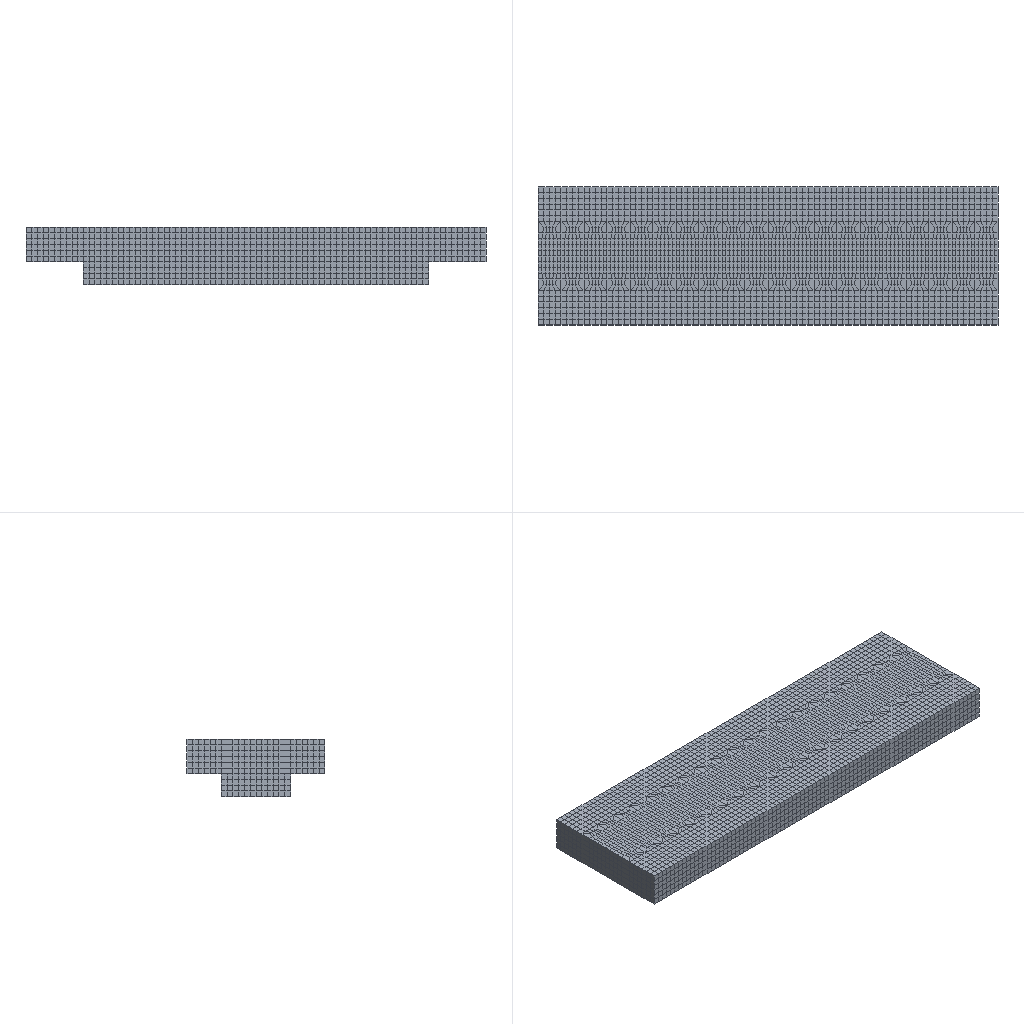Simulation study | abaqus
Set-up summary:
category,name,step,type,value,unit,region
solver,abaqus
solver,version,,,Abaqus/Standard 2020
units,not stated in the deck,,not stated
analysis,deck,,coupled temperature-displacement,coupled temperature-displacement
load_step,Step-1,Step-1,coupled temperature-displacement,nlgeom=True
contact,interactions,,,general=0 pairs=1 ties=0
load_step,requested,,,1
mesh,nodes,,,20926
mesh,elements,,,16800
element_type,C3D8RT,,solid,16800
load,load commands in deck,,count,4
bc,support commands in deck,,count,8
material,TC4,,in results
check,setup vs results,,match,"per instance, exact: element labels, types and connectivity; labels of the nodes the elements use; coordinates of those nodes at SINGLE_PRECISION in 2 of 2 instance(s)"
Abaqus input file, long lists of numbers shortened:
*Heading
** Job name: Job-1 Model name: Model-1
** Generated by: Abaqus/CAE 2020
*Preprint, echo=NO, model=NO, history=NO, contact=NO
**
** PARTS
**
*Part, name=Part-1
*Node
      1,           0.,          -9.,           3.
      2,           0.,        -8.25,           3.
** (3963 more lines like these left out)
*Element, type=C3D8RT
   1,   66,   67,   80,   79,    1,    2,   15,   14
   2,   67,   68,   81,   80,    2,    3,   16,   15
** (2878 more lines like these left out)
*Nset, nset=Set-2, generate
    1,  3965,     1
*Elset, elset=Set-2, generate
    1,  2880,     1
** Section: Section-1
*Solid Section, elset=Set-2, material=tc4
,
*End Part
**
*Part, name=Part-2
*Node
      1,          60.,         -4.5,           0.
      2,         58.5,         -4.5,           0.
** (16959 more lines like these left out)
*Element, type=C3D8RT
   1,  687, 2301, 7847, 2251,    1,  381, 1461,  509
   2, 2301, 2302, 7848, 7847,  381,    2, 1462, 1461
** (13918 more lines like these left out)
*Nset, nset=Set-5, generate
     1,  16961,      1
*Elset, elset=Set-5, generate
     1,  13920,      1
** Section: Section-1
*Solid Section, elset=Set-5, material=tc4
,
*End Part
**
**
** ASSEMBLY
**
*Assembly, name=Assembly
**
*Instance, name=Part-1-1, part=Part-1
         7.5,         -4.5,          -3.
*End Instance
**
*Instance, name=Part-2-1, part=Part-2
*End Instance
**
*Node
      1,          30.,          -9.,          -3.
*Nset, nset=Set-1, instance=Part-2-1
   44,   45,   46,   47,  210,  211,  212,  213,  214,  217,  218,  260,  510,  511,  512,  513
  514,  515,  516,  517,  518,  519,  520,  521,  522,  523,  524,  525,  526,  527,  528,  529
** (150 more lines like these left out)
*Elset, elset=Set-1, instance=Part-2-1
  2401,  2402,  2403,  2404,  2405,  2406,  2407,  2408,  2409,  2410,  2411,  2412,  2413,  2414,  2415,  2416
  2417,  2418,  2419,  2420,  2421,  2422,  2423,  2424,  2425,  2426,  2427,  2428,  2429,  2430,  2431,  2432
** (143 more lines like these left out)
*Nset, nset=Set-2, instance=Part-1-1, generate
    1,  3965,     1
*Nset, nset=Set-2, instance=Part-2-1, generate
     1,  16961,      1
*Elset, elset=Set-2, instance=Part-1-1, generate
    1,  2880,     1
*Elset, elset=Set-2, instance=Part-2-1, generate
     1,  13920,      1
*Nset, nset=Set-4
 1,
*Nset, nset=m_Set-3
 1,
*Elset, elset=_Surf-3_S1, internal, instance=Part-1-1, generate
 2833,  2880,     1
*Elset, elset=_Surf-3_S1, internal, instance=Part-2-1
  2401,  2402,  2403,  2404,  2405,  2406,  2407,  2408,  2409,  2410,  2411,  2412,  2413,  2414,  2415,  2416
  2417,  2418,  2419,  2420,  2421,  2422,  2423,  2424,  2425,  2426,  2427,  2428,  2429,  2430,  2431,  2432
** (113 more lines like these left out)
*Elset, elset=_Surf-3_S6, internal, instance=Part-1-1, generate
    1,  2869,    12
*Elset, elset=_Surf-3_S6, internal, instance=Part-2-1
     1,    81,   161,   241,   321,   401,   481,   561,   641,   721,   801,   881,   961,  1041,  1121,  1201
  1281,  1361,  1441,  1521,  1601,  1681,  1761,  1841,  1921,  2001,  2081,  2161,  2241,  2321,  2401,  2481
** (32 more lines like these left out)
*Elset, elset=_Surf-3_S2, internal, instance=Part-1-1, generate
  1,  48,   1
*Elset, elset=_Surf-3_S2, internal, instance=Part-2-1
     1,     2,     3,     4,     5,     6,     7,     8,     9,    10,    11,    12,    13,    14,    15,    16
    17,    18,    19,    20,    21,    22,    23,    24,    25,    26,    27,    28,    29,    30,    31,    32
** (143 more lines like these left out)
*Elset, elset=_Surf-3_S4, internal, instance=Part-1-1, generate
   12,  2880,    12
*Elset, elset=_Surf-3_S4, internal, instance=Part-2-1
    80,   160,   240,   320,   400,   480,   560,   640,   720,   800,   880,   960,  1040,  1120,  1200,  1280
  1360,  1440,  1520,  1600,  1680,  1760,  1840,  1920,  2000,  2080,  2160,  2240,  2320,  2400,  2480,  2560
** (31 more lines like these left out)
*Elset, elset=_Surf-3_S3, internal, instance=Part-1-1
    1,    2,    3,    4,    5,    6,    7,    8,    9,   10,   11,   12,   49,   50,   51,   52
   53,   54,   55,   56,   57,   58,   59,   60,   97,   98,   99,  100,  101,  102,  103,  104
** (43 more lines like these left out)
*Elset, elset=_Surf-3_S3, internal, instance=Part-2-1
  2881,  2882,  2883,  2884,  2885,  2886,  2887,  2888,  3841,  3842,  3843,  3844,  3845,  3846,  3847,  3848
  4801,  4802,  4803,  4804,  4805,  4806,  4807,  4808,  5761,  5762,  5763,  5764,  5765,  5766,  5767,  5768
** (4 more lines like these left out)
*Elset, elset=_Surf-3_S5, internal, instance=Part-1-1
   37,   38,   39,   40,   41,   42,   43,   44,   45,   46,   47,   48,   85,   86,   87,   88
   89,   90,   91,   92,   93,   94,   95,   96,  133,  134,  135,  136,  137,  138,  139,  140
** (43 more lines like these left out)
*Elset, elset=_Surf-3_S5, internal, instance=Part-2-1
   401,   402,   403,   404,   405,   406,   407,   408,   409,   410,   411,   412,   413,   414,   415,   416
   417,   418,   419,   420,   421,   422,   423,   424,   425,   426,   427,   428,   429,   430,   431,   432
** (34 more lines like these left out)
*Surface, type=ELEMENT, name=Surf-3
_Surf-3_S1, S1
_Surf-3_S6, S6
_Surf-3_S2, S2
_Surf-3_S4, S4
_Surf-3_S3, S3
_Surf-3_S5, S5
*Elset, elset=_Surf-4_S1, internal, instance=Part-1-1, generate
 2833,  2880,     1
*Elset, elset=_Surf-4_S1, internal, instance=Part-2-1
  2401,  2402,  2403,  2404,  2405,  2406,  2407,  2408,  2409,  2410,  2411,  2412,  2413,  2414,  2415,  2416
  2417,  2418,  2419,  2420,  2421,  2422,  2423,  2424,  2425,  2426,  2427,  2428,  2429,  2430,  2431,  2432
** (113 more lines like these left out)
*Elset, elset=_Surf-4_S6, internal, instance=Part-1-1, generate
    1,  2869,    12
*Elset, elset=_Surf-4_S6, internal, instance=Part-2-1
     1,    81,   161,   241,   321,   401,   481,   561,   641,   721,   801,   881,   961,  1041,  1121,  1201
  1281,  1361,  1441,  1521,  1601,  1681,  1761,  1841,  1921,  2001,  2081,  2161,  2241,  2321,  2401,  2481
** (32 more lines like these left out)
*Elset, elset=_Surf-4_S2, internal, instance=Part-1-1, generate
  1,  48,   1
*Elset, elset=_Surf-4_S2, internal, instance=Part-2-1
     1,     2,     3,     4,     5,     6,     7,     8,     9,    10,    11,    12,    13,    14,    15,    16
    17,    18,    19,    20,    21,    22,    23,    24,    25,    26,    27,    28,    29,    30,    31,    32
** (143 more lines like these left out)
*Elset, elset=_Surf-4_S4, internal, instance=Part-1-1, generate
   12,  2880,    12
*Elset, elset=_Surf-4_S4, internal, instance=Part-2-1
    80,   160,   240,   320,   400,   480,   560,   640,   720,   800,   880,   960,  1040,  1120,  1200,  1280
  1360,  1440,  1520,  1600,  1680,  1760,  1840,  1920,  2000,  2080,  2160,  2240,  2320,  2400,  2480,  2560
** (31 more lines like these left out)
*Elset, elset=_Surf-4_S3, internal, instance=Part-1-1
    1,    2,    3,    4,    5,    6,    7,    8,    9,   10,   11,   12,   49,   50,   51,   52
   53,   54,   55,   56,   57,   58,   59,   60,   97,   98,   99,  100,  101,  102,  103,  104
** (43 more lines like these left out)
*Elset, elset=_Surf-4_S3, internal, instance=Part-2-1
  2881,  2882,  2883,  2884,  2885,  2886,  2887,  2888,  3841,  3842,  3843,  3844,  3845,  3846,  3847,  3848
  4801,  4802,  4803,  4804,  4805,  4806,  4807,  4808,  5761,  5762,  5763,  5764,  5765,  5766,  5767,  5768
** (4 more lines like these left out)
*Elset, elset=_Surf-4_S5, internal, instance=Part-1-1
   37,   38,   39,   40,   41,   42,   43,   44,   45,   46,   47,   48,   85,   86,   87,   88
   89,   90,   91,   92,   93,   94,   95,   96,  133,  134,  135,  136,  137,  138,  139,  140
** (43 more lines like these left out)
*Elset, elset=_Surf-4_S5, internal, instance=Part-2-1
   401,   402,   403,   404,   405,   406,   407,   408,   409,   410,   411,   412,   413,   414,   415,   416
   417,   418,   419,   420,   421,   422,   423,   424,   425,   426,   427,   428,   429,   430,   431,   432
** (34 more lines like these left out)
*Surface, type=ELEMENT, name=Surf-4
_Surf-4_S1, S1
_Surf-4_S6, S6
_Surf-4_S2, S2
_Surf-4_S4, S4
_Surf-4_S3, S3
_Surf-4_S5, S5
*Elset, elset=_Surf-6_S5, internal, instance=Part-1-1
   37,   38,   39,   40,   41,   42,   43,   44,   45,   46,   47,   48,   85,   86,   87,   88
   89,   90,   91,   92,   93,   94,   95,   96,  133,  134,  135,  136,  137,  138,  139,  140
** (43 more lines like these left out)
*Surface, type=ELEMENT, name=Surf-6
_Surf-6_S5, S5
*Elset, elset=_m_Surf-1_S3, internal, instance=Part-1-1
    1,    2,    3,    4,    5,    6,    7,    8,    9,   10,   11,   12,   49,   50,   51,   52
   53,   54,   55,   56,   57,   58,   59,   60,   97,   98,   99,  100,  101,  102,  103,  104
** (43 more lines like these left out)
*Surface, type=ELEMENT, name=m_Surf-1
_m_Surf-1_S3, S3
*Elset, elset=_s_Surf-1_S4, internal, instance=Part-2-1, generate
  8646,  11520,      6
*Elset, elset=_s_Surf-1_S1, internal, instance=Part-2-1
 11521, 11522, 11523, 11524, 11525, 11526, 11527, 11528, 11529, 11530, 11531, 11532, 11533, 11534, 11535, 11536
 11537, 11538, 11539, 11540, 11541, 11542, 11543, 11544, 11545, 11546, 11547, 11548, 11549, 11550, 11551, 11552
** (23 more lines like these left out)
*Elset, elset=_s_Surf-1_S2, internal, instance=Part-2-1
    1,    2,    3,    4,    5,    6,    7,    8,    9,   10,   11,   12,   13,   14,   15,   16
   17,   18,   19,   20,   21,   22,   23,   24,   25,   26,   27,   28,   29,   30,   31,   32
** (88 more lines like these left out)
*Surface, type=ELEMENT, name=s_Surf-1
_s_Surf-1_S4, S4
_s_Surf-1_S1, S1
_s_Surf-1_S2, S2
*Elset, elset=_s_Surf-5_S5, internal, instance=Part-1-1
   37,   38,   39,   40,   41,   42,   43,   44,   45,   46,   47,   48,   85,   86,   87,   88
   89,   90,   91,   92,   93,   94,   95,   96,  133,  134,  135,  136,  137,  138,  139,  140
** (43 more lines like these left out)
*Surface, type=ELEMENT, name=s_Surf-5
_s_Surf-5_S5, S5
** Constraint: Constraint-1
*Coupling, constraint name=Constraint-1, ref node=m_Set-3, surface=s_Surf-5
*Kinematic
*End Assembly
*Amplitude, name=Amp-1, definition=PERIODIC
1,            62.8,              0.,              0.
            0.1,              0.
**
** MATERIALS
**
*Material, name=tc4
*Conductivity
  7.5, 20.
  8.7,200.
 11.8,500.
*Density
 4.4e-09,
*Elastic
108000., 0.33
*Expansion
 9.1e-06, 20.
 9.2e-06,250.
 9.7e-06,500.
*Plastic, hardening=JOHNSON COOK
860., 683., 0.47,   1.,1650.,  25.
*Rate Dependent, type=JOHNSON COOK
 0.035,1.
*Specific Heat
 5.263e+08,
**
** INTERACTION PROPERTIES
**
*Surface Interaction, name=IntProp-1
1.,
*Friction, slip tolerance=0.005
 0.15,
*Surface Behavior, pressure-overclosure=HARD
*Gap Conductance
11.,  0.
 0., 0.1
**
** PHYSICAL CONSTANTS
**
*Physical Constants, absolute zero=-273., stefan boltzmann=5.67e-08
**
** PREDEFINED FIELDS
**
** Name: Predefined Field-1   Type: Temperature
*Initial Conditions, type=TEMPERATURE
Set-2, 25.
**
** INTERACTIONS
**
** Interaction: Int-1
*Contact Pair, interaction=IntProp-1, type=SURFACE TO SURFACE
s_Surf-1, m_Surf-1
** ----------------------------------------------------------------
**
** STEP: Step-1
**
*Step, name=Step-1, nlgeom=YES, inc=10000
*Coupled Temperature-displacement, creep=none, deltmx=1e+09, stabilize=0.0002, allsdtol=0.05, continue=NO
0.1, 11., 0.00011, 0.25
**
** BOUNDARY CONDITIONS
**
** Name: BC-1 Type: 对称/反对称/完全固定
*Boundary
Set-1, ENCASTRE
** Name: BC-2 Type: 位移/转角
*Boundary
Set-4, 1, 1, 1.
Set-4, 2, 2
Set-4, 4, 4
Set-4, 5, 5
Set-4, 6, 6
**
** LOADS
**
** Name: Load-1   Type: Pressure
*Dsload
Surf-6, P, 5.
**
** INTERACTIONS
**
** Interaction: Int-2
*Sfilm
Surf-3, F, 25., 0.05
** Interaction: Int-3
*Sradiate
Surf-4, AVG, 0.0, 0.6
**
** OUTPUT REQUESTS
**
*Restart, write, frequency=0
**
** FIELD OUTPUT: F-Output-1
**
*Output, field
*Node Output
CF, NT, RF, RFL, RM, RT, U, V
*Element Output, directions=YES
E, HFL, LE, MISES, MISESMAX, MISESONLY, PE, PEEQ, PEEQMAX, PEEQT, PEMAG, S, SSAVG, TEMP, YIELDPOT
*Contact Output
CDISP, CSTRESS
*Radiation Output
FTEMP,
**
** HISTORY OUTPUT: H-Output-1
**
*Output, history, variable=PRESELECT
*End Step
Results summary:
result,step,,completed,increments=47 time=11.0/11.0
result,analysis,,,"coupled temperature-displacement, steady state"
result,last_loadstep,,,1
result,analysis steps,,count,1
result,primary field,,,"U, NT11"
result,reaction total,,FX,1.3e-05,model units
result,reaction total,,FY,-0.0,model units
result,reaction total,,FZ,-2025,model units